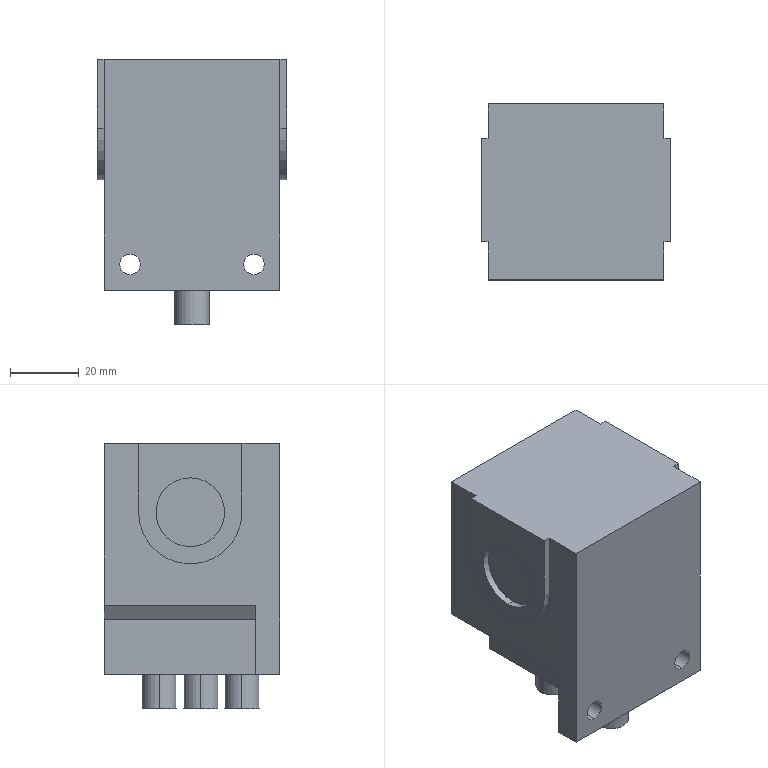Part | STEP file | Limit Switch | 1 solid | 40 faces | box 55 x 51 x 77 mm | volume 154232 mm3 | plane 23 | cylinder 17 | commonest cylinder face diameters 10 x6 6 x4 20 x4 30 x3
STEP:
#1=CARTESIAN_POINT('',(-18.,7.,-7.241));
#2=VERTEX_POINT('',#1);
#3=CARTESIAN_POINT('',(-18.,7.,-13.241));
#4=VERTEX_POINT('',#3);
#5=CARTESIAN_POINT('',(-18.,7.,-10.241));
#6=DIRECTION('',(0.,-1.,0.));
#7=DIRECTION('',(0.,0.,-1.));
#8=AXIS2_PLACEMENT_3D('',#5,#6,#7);
#9=CIRCLE('',#8,3.);
#10=EDGE_CURVE('',#2,#4,#9,.T.);
#11=ORIENTED_EDGE('',*,*,#10,.F.);
#12=CARTESIAN_POINT('',(-18.,0.,-7.241));
#13=VERTEX_POINT('',#12);
#14=CARTESIAN_POINT('',(-18.,44.,-7.241));
#15=DIRECTION('',(0.,-1.,0.));
#16=VECTOR('',#15,1000.);
#17=LINE('',#14,#16);
#18=EDGE_CURVE('',#2,#13,#17,.T.);
#19=ORIENTED_EDGE('',*,*,#18,.T.);
#20=CARTESIAN_POINT('',(-18.,0.,-13.241));
#21=VERTEX_POINT('',#20);
#22=CARTESIAN_POINT('',(-18.,0.,-10.241));
#23=DIRECTION('',(0.,-1.,0.));
#24=DIRECTION('',(0.,0.,-1.));
#25=AXIS2_PLACEMENT_3D('',#22,#23,#24);
#26=CIRCLE('',#25,3.);
#27=EDGE_CURVE('',#13,#21,#26,.T.);
#28=ORIENTED_EDGE('',*,*,#27,.T.);
#29=CARTESIAN_POINT('',(-18.,44.,-13.241));
#30=DIRECTION('',(0.,-1.,0.));
#31=VECTOR('',#30,1000.);
#32=LINE('',#29,#31);
#33=EDGE_CURVE('',#4,#21,#32,.T.);
#34=ORIENTED_EDGE('',*,*,#33,.F.);
#35=EDGE_LOOP('',(#11,#19,#28,#34));
#36=FACE_OUTER_BOUND('',#35,.T.);
#37=CARTESIAN_POINT('',(-18.,44.,-10.241));
#38=DIRECTION('',(0.,-1.,0.));
#39=DIRECTION('',(0.,0.,-1.));
#40=AXIS2_PLACEMENT_3D('',#37,#38,#39);
#41=CYLINDRICAL_SURFACE('',#40,3.);
#42=ADVANCED_FACE('',(#36),#41,.F.);
#43=CARTESIAN_POINT('',(18.,7.,-7.241));
#44=VERTEX_POINT('',#43);
#45=CARTESIAN_POINT('',(18.,7.,-13.241));
#46=VERTEX_POINT('',#45);
#47=CARTESIAN_POINT('',(18.,7.,-10.241));
#48=DIRECTION('',(0.,-1.,0.));
#49=DIRECTION('',(0.,0.,-1.));
#50=AXIS2_PLACEMENT_3D('',#47,#48,#49);
#51=CIRCLE('',#50,3.);
#52=EDGE_CURVE('',#44,#46,#51,.T.);
#53=ORIENTED_EDGE('',*,*,#52,.F.);
#54=CARTESIAN_POINT('',(18.,0.,-7.241));
#55=VERTEX_POINT('',#54);
#56=CARTESIAN_POINT('',(18.,44.,-7.241));
#57=DIRECTION('',(0.,-1.,0.));
#58=VECTOR('',#57,1000.);
#59=LINE('',#56,#58);
#60=EDGE_CURVE('',#44,#55,#59,.T.);
#61=ORIENTED_EDGE('',*,*,#60,.T.);
#62=CARTESIAN_POINT('',(18.,0.,-13.241));
#63=VERTEX_POINT('',#62);
#64=CARTESIAN_POINT('',(18.,0.,-10.241));
#65=DIRECTION('',(0.,-1.,0.));
#66=DIRECTION('',(0.,0.,-1.));
#67=AXIS2_PLACEMENT_3D('',#64,#65,#66);
#68=CIRCLE('',#67,3.);
#69=EDGE_CURVE('',#55,#63,#68,.T.);
#70=ORIENTED_EDGE('',*,*,#69,.T.);
#71=CARTESIAN_POINT('',(18.,44.,-13.241));
#72=DIRECTION('',(0.,-1.,0.));
#73=VECTOR('',#72,1000.);
#74=LINE('',#71,#73);
#75=EDGE_CURVE('',#46,#63,#74,.T.);
#76=ORIENTED_EDGE('',*,*,#75,.F.);
#77=EDGE_LOOP('',(#53,#61,#70,#76));
#78=FACE_OUTER_BOUND('',#77,.T.);
#79=CARTESIAN_POINT('',(18.,44.,-10.241));
#80=DIRECTION('',(0.,-1.,0.));
#81=DIRECTION('',(0.,0.,-1.));
#82=AXIS2_PLACEMENT_3D('',#79,#80,#81);
#83=CYLINDRICAL_SURFACE('',#82,3.);
#84=ADVANCED_FACE('',(#78),#83,.F.);
#85=CARTESIAN_POINT('',(-27.5,11.,29.259));
#86=VERTEX_POINT('',#85);
#87=CARTESIAN_POINT('',(-27.5,26.,14.259));
#88=VERTEX_POINT('',#87);
#89=CARTESIAN_POINT('',(-27.5,26.,29.259));
#90=DIRECTION('',(1.,0.,0.));
#91=DIRECTION('',(0.,0.,-1.));
#92=AXIS2_PLACEMENT_3D('',#89,#90,#91);
#93=CIRCLE('',#92,15.);
#94=EDGE_CURVE('',#86,#88,#93,.T.);
#95=ORIENTED_EDGE('',*,*,#94,.T.);
#96=CARTESIAN_POINT('',(-25.5,26.,14.259));
#97=VERTEX_POINT('',#96);
#98=CARTESIAN_POINT('',(-27.5,26.,14.259));
#99=DIRECTION('',(1.,0.,0.));
#100=VECTOR('',#99,1000.);
#101=LINE('',#98,#100);
#102=EDGE_CURVE('',#88,#97,#101,.T.);
#103=ORIENTED_EDGE('',*,*,#102,.T.);
#104=CARTESIAN_POINT('',(-25.5,11.,29.259));
#105=VERTEX_POINT('',#104);
#106=CARTESIAN_POINT('',(-25.5,26.,29.259));
#107=DIRECTION('',(-1.,0.,0.));
#108=DIRECTION('',(0.,0.,-1.));
#109=AXIS2_PLACEMENT_3D('',#106,#107,#108);
#110=CIRCLE('',#109,15.);
#111=EDGE_CURVE('',#97,#105,#110,.T.);
#112=ORIENTED_EDGE('',*,*,#111,.T.);
#113=CARTESIAN_POINT('',(-27.5,11.,29.259));
#114=DIRECTION('',(-1.,0.,0.));
#115=VECTOR('',#114,1000.);
#116=LINE('',#113,#115);
#117=EDGE_CURVE('',#105,#86,#116,.T.);
#118=ORIENTED_EDGE('',*,*,#117,.T.);
#119=EDGE_LOOP('',(#95,#103,#112,#118));
#120=FACE_OUTER_BOUND('',#119,.T.);
#121=CARTESIAN_POINT('',(-27.5,26.,29.259));
#122=DIRECTION('',(1.,0.,0.));
#123=DIRECTION('',(0.,0.,-1.));
#124=AXIS2_PLACEMENT_3D('',#121,#122,#123);
#125=CYLINDRICAL_SURFACE('',#124,15.);
#126=ADVANCED_FACE('',(#120),#125,.T.);
#127=CARTESIAN_POINT('',(5.,11.,-27.741));
#128=VERTEX_POINT('',#127);
#129=CARTESIAN_POINT('',(-5.,11.,-27.741));
#130=VERTEX_POINT('',#129);
#131=CARTESIAN_POINT('',(0.,11.,-27.741));
#132=DIRECTION('',(0.,0.,1.));
#133=DIRECTION('',(1.,0.,0.));
#134=AXIS2_PLACEMENT_3D('',#131,#132,#133);
#135=CIRCLE('',#134,5.);
#136=EDGE_CURVE('',#128,#130,#135,.T.);
#137=ORIENTED_EDGE('',*,*,#136,.T.);
#138=CARTESIAN_POINT('',(-5.,11.,-17.741));
#139=VERTEX_POINT('',#138);
#140=CARTESIAN_POINT('',(-5.,11.,-27.741));
#141=DIRECTION('',(0.,0.,1.));
#142=VECTOR('',#141,1000.);
#143=LINE('',#140,#142);
#144=EDGE_CURVE('',#130,#139,#143,.T.);
#145=ORIENTED_EDGE('',*,*,#144,.T.);
#146=CARTESIAN_POINT('',(5.,11.,-17.741));
#147=VERTEX_POINT('',#146);
#148=CARTESIAN_POINT('',(0.,11.,-17.741));
#149=DIRECTION('',(0.,0.,-1.));
#150=DIRECTION('',(1.,0.,0.));
#151=AXIS2_PLACEMENT_3D('',#148,#149,#150);
#152=CIRCLE('',#151,5.);
#153=EDGE_CURVE('',#139,#147,#152,.T.);
#154=ORIENTED_EDGE('',*,*,#153,.T.);
#155=CARTESIAN_POINT('',(5.,11.,-27.741));
#156=DIRECTION('',(0.,0.,1.));
#157=VECTOR('',#156,1000.);
#158=LINE('',#155,#157);
#159=EDGE_CURVE('',#128,#147,#158,.T.);
#160=ORIENTED_EDGE('',*,*,#159,.F.);
#161=EDGE_LOOP('',(#137,#145,#154,#160));
#162=FACE_OUTER_BOUND('',#161,.T.);
#163=CARTESIAN_POINT('',(0.,11.,-27.741));
#164=DIRECTION('',(0.,0.,1.));
#165=DIRECTION('',(1.,0.,0.));
#166=AXIS2_PLACEMENT_3D('',#163,#164,#165);
#167=CYLINDRICAL_SURFACE('',#166,5.);
#168=ADVANCED_FACE('',(#162),#167,.T.);
#169=CARTESIAN_POINT('',(5.,35.,-27.741));
#170=VERTEX_POINT('',#169);
#171=CARTESIAN_POINT('',(-5.,35.,-27.741));
#172=VERTEX_POINT('',#171);
#173=CARTESIAN_POINT('',(0.,35.,-27.741));
#174=DIRECTION('',(0.,0.,1.));
#175=DIRECTION('',(1.,0.,0.));
#176=AXIS2_PLACEMENT_3D('',#173,#174,#175);
#177=CIRCLE('',#176,5.);
#178=EDGE_CURVE('',#170,#172,#177,.T.);
#179=ORIENTED_EDGE('',*,*,#178,.T.);
#180=CARTESIAN_POINT('',(-5.,35.,-17.741));
#181=VERTEX_POINT('',#180);
#182=CARTESIAN_POINT('',(-5.,35.,-27.741));
#183=DIRECTION('',(0.,0.,1.));
#184=VECTOR('',#183,1000.);
#185=LINE('',#182,#184);
#186=EDGE_CURVE('',#172,#181,#185,.T.);
#187=ORIENTED_EDGE('',*,*,#186,.T.);
#188=CARTESIAN_POINT('',(5.,35.,-17.741));
#189=VERTEX_POINT('',#188);
#190=CARTESIAN_POINT('',(0.,35.,-17.741));
#191=DIRECTION('',(0.,0.,-1.));
#192=DIRECTION('',(1.,0.,0.));
#193=AXIS2_PLACEMENT_3D('',#190,#191,#192);
#194=CIRCLE('',#193,5.);
#195=EDGE_CURVE('',#181,#189,#194,.T.);
#196=ORIENTED_EDGE('',*,*,#195,.T.);
#197=CARTESIAN_POINT('',(5.,35.,-27.741));
#198=DIRECTION('',(0.,0.,1.));
#199=VECTOR('',#198,1000.);
#200=LINE('',#197,#199);
#201=EDGE_CURVE('',#170,#189,#200,.T.);
#202=ORIENTED_EDGE('',*,*,#201,.F.);
#203=EDGE_LOOP('',(#179,#187,#196,#202));
#204=FACE_OUTER_BOUND('',#203,.T.);
#205=CARTESIAN_POINT('',(0.,35.,-27.741));
#206=DIRECTION('',(0.,0.,1.));
#207=DIRECTION('',(1.,0.,0.));
#208=AXIS2_PLACEMENT_3D('',#205,#206,#207);
#209=CYLINDRICAL_SURFACE('',#208,5.);
#210=ADVANCED_FACE('',(#204),#209,.T.);
#211=CARTESIAN_POINT('',(5.,23.,-27.741));
#212=VERTEX_POINT('',#211);
#213=CARTESIAN_POINT('',(-5.,23.,-27.741));
#214=VERTEX_POINT('',#213);
#215=CARTESIAN_POINT('',(0.,23.,-27.741));
#216=DIRECTION('',(0.,0.,1.));
#217=DIRECTION('',(1.,0.,0.));
#218=AXIS2_PLACEMENT_3D('',#215,#216,#217);
#219=CIRCLE('',#218,5.);
#220=EDGE_CURVE('',#212,#214,#219,.T.);
#221=ORIENTED_EDGE('',*,*,#220,.T.);
#222=CARTESIAN_POINT('',(-5.,23.,-17.741));
#223=VERTEX_POINT('',#222);
#224=CARTESIAN_POINT('',(-5.,23.,-27.741));
#225=DIRECTION('',(0.,0.,1.));
#226=VECTOR('',#225,1000.);
#227=LINE('',#224,#226);
#228=EDGE_CURVE('',#214,#223,#227,.T.);
#229=ORIENTED_EDGE('',*,*,#228,.T.);
#230=CARTESIAN_POINT('',(5.,23.,-17.741));
#231=VERTEX_POINT('',#230);
#232=CARTESIAN_POINT('',(0.,23.,-17.741));
#233=DIRECTION('',(0.,0.,-1.));
#234=DIRECTION('',(1.,0.,0.));
#235=AXIS2_PLACEMENT_3D('',#232,#233,#234);
#236=CIRCLE('',#235,5.);
#237=EDGE_CURVE('',#223,#231,#236,.T.);
#238=ORIENTED_EDGE('',*,*,#237,.T.);
#239=CARTESIAN_POINT('',(5.,23.,-27.741));
#240=DIRECTION('',(0.,0.,1.));
#241=VECTOR('',#240,1000.);
#242=LINE('',#239,#241);
#243=EDGE_CURVE('',#212,#231,#242,.T.);
#244=ORIENTED_EDGE('',*,*,#243,.F.);
#245=EDGE_LOOP('',(#221,#229,#238,#244));
#246=FACE_OUTER_BOUND('',#245,.T.);
#247=CARTESIAN_POINT('',(0.,23.,-27.741));
#248=DIRECTION('',(0.,0.,1.));
#249=DIRECTION('',(1.,0.,0.));
#250=AXIS2_PLACEMENT_3D('',#247,#248,#249);
#251=CYLINDRICAL_SURFACE('',#250,5.);
#252=ADVANCED_FACE('',(#246),#251,.T.);
#253=CARTESIAN_POINT('',(27.5,26.,19.259));
#254=VERTEX_POINT('',#253);
#255=CARTESIAN_POINT('',(27.5,26.,39.259));
#256=VERTEX_POINT('',#255);
#257=CARTESIAN_POINT('',(27.5,26.,29.259));
#258=DIRECTION('',(-1.,0.,0.));
#259=DIRECTION('',(0.,0.,1.));
#260=AXIS2_PLACEMENT_3D('',#257,#258,#259);
#261=CIRCLE('',#260,10.);
#262=EDGE_CURVE('',#254,#256,#261,.T.);
#263=ORIENTED_EDGE('',*,*,#262,.F.);
#264=CARTESIAN_POINT('',(25.5,26.,19.259));
#265=VERTEX_POINT('',#264);
#266=CARTESIAN_POINT('',(27.5,26.,19.259));
#267=DIRECTION('',(-1.,0.,0.));
#268=VECTOR('',#267,1000.);
#269=LINE('',#266,#268);
#270=EDGE_CURVE('',#254,#265,#269,.T.);
#271=ORIENTED_EDGE('',*,*,#270,.T.);
#272=CARTESIAN_POINT('',(25.5,26.,39.259));
#273=VERTEX_POINT('',#272);
#274=CARTESIAN_POINT('',(25.5,26.,29.259));
#275=DIRECTION('',(1.,0.,0.));
#276=DIRECTION('',(0.,0.,1.));
#277=AXIS2_PLACEMENT_3D('',#274,#275,#276);
#278=CIRCLE('',#277,10.);
#279=EDGE_CURVE('',#273,#265,#278,.T.);
#280=ORIENTED_EDGE('',*,*,#279,.F.);
#281=CARTESIAN_POINT('',(27.5,26.,39.259));
#282=DIRECTION('',(-1.,0.,0.));
#283=VECTOR('',#282,1000.);
#284=LINE('',#281,#283);
#285=EDGE_CURVE('',#256,#273,#284,.T.);
#286=ORIENTED_EDGE('',*,*,#285,.F.);
#287=EDGE_LOOP('',(#263,#271,#280,#286));
#288=FACE_OUTER_BOUND('',#287,.T.);
#289=CARTESIAN_POINT('',(27.5,26.,29.259));
#290=DIRECTION('',(-1.,0.,0.));
#291=DIRECTION('',(0.,0.,1.));
#292=AXIS2_PLACEMENT_3D('',#289,#290,#291);
#293=CYLINDRICAL_SURFACE('',#292,10.);
#294=ADVANCED_FACE('',(#288),#293,.F.);
#295=CARTESIAN_POINT('',(-27.5,26.,39.259));
#296=VERTEX_POINT('',#295);
#297=CARTESIAN_POINT('',(-27.5,26.,19.259));
#298=VERTEX_POINT('',#297);
#299=CARTESIAN_POINT('',(-27.5,26.,29.259));
#300=DIRECTION('',(1.,0.,0.));
#301=DIRECTION('',(0.,0.,-1.));
#302=AXIS2_PLACEMENT_3D('',#299,#300,#301);
#303=CIRCLE('',#302,10.);
#304=EDGE_CURVE('',#296,#298,#303,.T.);
#305=ORIENTED_EDGE('',*,*,#304,.F.);
#306=CARTESIAN_POINT('',(-25.5,26.,39.259));
#307=VERTEX_POINT('',#306);
#308=CARTESIAN_POINT('',(-27.5,26.,39.259));
#309=DIRECTION('',(1.,0.,0.));
#310=VECTOR('',#309,1000.);
#311=LINE('',#308,#310);
#312=EDGE_CURVE('',#296,#307,#311,.T.);
#313=ORIENTED_EDGE('',*,*,#312,.T.);
#314=CARTESIAN_POINT('',(-25.5,26.,19.259));
#315=VERTEX_POINT('',#314);
#316=CARTESIAN_POINT('',(-25.5,26.,29.259));
#317=DIRECTION('',(-1.,0.,0.));
#318=DIRECTION('',(0.,0.,-1.));
#319=AXIS2_PLACEMENT_3D('',#316,#317,#318);
#320=CIRCLE('',#319,10.);
#321=EDGE_CURVE('',#315,#307,#320,.T.);
#322=ORIENTED_EDGE('',*,*,#321,.F.);
#323=CARTESIAN_POINT('',(-27.5,26.,19.259));
#324=DIRECTION('',(1.,0.,0.));
#325=VECTOR('',#324,1000.);
#326=LINE('',#323,#325);
#327=EDGE_CURVE('',#298,#315,#326,.T.);
#328=ORIENTED_EDGE('',*,*,#327,.F.);
#329=EDGE_LOOP('',(#305,#313,#322,#328));
#330=FACE_OUTER_BOUND('',#329,.T.);
#331=CARTESIAN_POINT('',(-27.5,26.,29.259));
#332=DIRECTION('',(1.,0.,0.));
#333=DIRECTION('',(0.,0.,-1.));
#334=AXIS2_PLACEMENT_3D('',#331,#332,#333);
#335=CYLINDRICAL_SURFACE('',#334,10.);
#336=ADVANCED_FACE('',(#330),#335,.F.);
#337=CARTESIAN_POINT('',(25.5,0.,-17.741));
#338=VERTEX_POINT('',#337);
#339=CARTESIAN_POINT('',(-25.5,0.,-17.741));
#340=VERTEX_POINT('',#339);
#341=CARTESIAN_POINT('',(0.,0.,-17.741));
#342=DIRECTION('',(-1.,0.,0.));
#343=VECTOR('',#342,1000.);
#344=LINE('',#341,#343);
#345=EDGE_CURVE('',#338,#340,#344,.T.);
#346=ORIENTED_EDGE('',*,*,#345,.F.);
#347=CARTESIAN_POINT('',(25.5,0.,49.259));
#348=VERTEX_POINT('',#347);
#349=CARTESIAN_POINT('',(25.5,0.,0.));
#350=DIRECTION('',(0.,0.,-1.));
#351=VECTOR('',#350,1000.);
#352=LINE('',#349,#351);
#353=EDGE_CURVE('',#348,#338,#352,.T.);
#354=ORIENTED_EDGE('',*,*,#353,.F.);
#355=CARTESIAN_POINT('',(-25.5,0.,49.259));
#356=VERTEX_POINT('',#355);
#357=CARTESIAN_POINT('',(0.,0.,49.259));
#358=DIRECTION('',(1.,0.,0.));
#359=VECTOR('',#358,1000.);
#360=LINE('',#357,#359);
#361=EDGE_CURVE('',#356,#348,#360,.T.);
#362=ORIENTED_EDGE('',*,*,#361,.F.);
#363=CARTESIAN_POINT('',(-25.5,0.,0.));
#364=DIRECTION('',(0.,0.,1.));
#365=VECTOR('',#364,1000.);
#366=LINE('',#363,#365);
#367=EDGE_CURVE('',#340,#356,#366,.T.);
#368=ORIENTED_EDGE('',*,*,#367,.F.);
#369=EDGE_LOOP('',(#346,#354,#362,#368));
#370=FACE_OUTER_BOUND('',#369,.T.);
#371=CARTESIAN_POINT('',(-18.,0.,-10.241));
#372=DIRECTION('',(0.,-1.,0.));
#373=DIRECTION('',(0.,0.,-1.));
#374=AXIS2_PLACEMENT_3D('',#371,#372,#373);
#375=CIRCLE('',#374,3.);
#376=EDGE_CURVE('',#21,#13,#375,.T.);
#377=ORIENTED_EDGE('',*,*,#376,.F.);
#378=ORIENTED_EDGE('',*,*,#27,.F.);
#379=EDGE_LOOP('',(#377,#378));
#380=FACE_BOUND('',#379,.T.);
#381=CARTESIAN_POINT('',(18.,0.,-10.241));
#382=DIRECTION('',(0.,-1.,0.));
#383=DIRECTION('',(0.,0.,-1.));
#384=AXIS2_PLACEMENT_3D('',#381,#382,#383);
#385=CIRCLE('',#384,3.);
#386=EDGE_CURVE('',#63,#55,#385,.T.);
#387=ORIENTED_EDGE('',*,*,#386,.F.);
#388=ORIENTED_EDGE('',*,*,#69,.F.);
#389=EDGE_LOOP('',(#387,#388));
#390=FACE_BOUND('',#389,.T.);
#391=CARTESIAN_POINT('',(0.,0.,0.));
#392=DIRECTION('',(0.,1.,0.));
#393=DIRECTION('',(0.,0.,1.));
#394=AXIS2_PLACEMENT_3D('',#391,#392,#393);
#395=PLANE('',#394);
#396=ADVANCED_FACE('',(#370,#380,#390),#395,.F.);
#397=CARTESIAN_POINT('',(-25.5,41.,29.259));
#398=VERTEX_POINT('',#397);
#399=CARTESIAN_POINT('',(-25.5,26.,29.259));
#400=DIRECTION('',(-1.,0.,0.));
#401=DIRECTION('',(0.,0.,-1.));
#402=AXIS2_PLACEMENT_3D('',#399,#400,#401);
#403=CIRCLE('',#402,15.);
#404=EDGE_CURVE('',#398,#97,#403,.T.);
#405=ORIENTED_EDGE('',*,*,#404,.F.);
#406=CARTESIAN_POINT('',(-25.5,41.,49.259));
#407=VERTEX_POINT('',#406);
#408=CARTESIAN_POINT('',(-25.5,41.,-17.741));
#409=DIRECTION('',(0.,0.,-1.));
#410=VECTOR('',#409,1000.);
#411=LINE('',#408,#410);
#412=EDGE_CURVE('',#407,#398,#411,.T.);
#413=ORIENTED_EDGE('',*,*,#412,.F.);
#414=CARTESIAN_POINT('',(-25.5,51.,49.259));
#415=VERTEX_POINT('',#414);
#416=CARTESIAN_POINT('',(-25.5,51.,49.259));
#417=DIRECTION('',(0.,-1.,0.));
#418=VECTOR('',#417,1000.);
#419=LINE('',#416,#418);
#420=EDGE_CURVE('',#415,#407,#419,.T.);
#421=ORIENTED_EDGE('',*,*,#420,.F.);
#422=CARTESIAN_POINT('',(-25.5,51.,2.259));
#423=VERTEX_POINT('',#422);
#424=CARTESIAN_POINT('',(-25.5,51.,-17.741));
#425=DIRECTION('',(0.,0.,1.));
#426=VECTOR('',#425,1000.);
#427=LINE('',#424,#426);
#428=EDGE_CURVE('',#423,#415,#427,.T.);
#429=ORIENTED_EDGE('',*,*,#428,.F.);
#430=CARTESIAN_POINT('',(-25.5,7.,2.259));
#431=VERTEX_POINT('',#430);
#432=CARTESIAN_POINT('',(-25.5,51.,2.259));
#433=DIRECTION('',(0.,1.,0.));
#434=VECTOR('',#433,1000.);
#435=LINE('',#432,#434);
#436=EDGE_CURVE('',#431,#423,#435,.T.);
#437=ORIENTED_EDGE('',*,*,#436,.F.);
#438=CARTESIAN_POINT('',(-25.5,7.,-17.741));
#439=VERTEX_POINT('',#438);
#440=CARTESIAN_POINT('',(-25.5,7.,-17.741));
#441=DIRECTION('',(0.,0.,1.));
#442=VECTOR('',#441,1000.);
#443=LINE('',#440,#442);
#444=EDGE_CURVE('',#439,#431,#443,.T.);
#445=ORIENTED_EDGE('',*,*,#444,.F.);
#446=CARTESIAN_POINT('',(-25.5,51.,-17.741));
#447=DIRECTION('',(0.,1.,0.));
#448=VECTOR('',#447,1000.);
#449=LINE('',#446,#448);
#450=EDGE_CURVE('',#340,#439,#449,.T.);
#451=ORIENTED_EDGE('',*,*,#450,.F.);
#452=ORIENTED_EDGE('',*,*,#367,.T.);
#453=CARTESIAN_POINT('',(-25.5,11.,49.259));
#454=VERTEX_POINT('',#453);
#455=CARTESIAN_POINT('',(-25.5,51.,49.259));
#456=DIRECTION('',(0.,-1.,0.));
#457=VECTOR('',#456,1000.);
#458=LINE('',#455,#457);
#459=EDGE_CURVE('',#454,#356,#458,.T.);
#460=ORIENTED_EDGE('',*,*,#459,.F.);
#461=CARTESIAN_POINT('',(-25.5,11.,-17.741));
#462=DIRECTION('',(0.,0.,1.));
#463=VECTOR('',#462,1000.);
#464=LINE('',#461,#463);
#465=EDGE_CURVE('',#105,#454,#464,.T.);
#466=ORIENTED_EDGE('',*,*,#465,.F.);
#467=ORIENTED_EDGE('',*,*,#111,.F.);
#468=EDGE_LOOP('',(#405,#413,#421,#429,#437,#445,#451,#452,#460,#466,#467));
#469=FACE_OUTER_BOUND('',#468,.T.);
#470=CARTESIAN_POINT('',(-25.5,51.,-17.741));
#471=DIRECTION('',(1.,0.,0.));
#472=DIRECTION('',(0.,0.,-1.));
#473=AXIS2_PLACEMENT_3D('',#470,#471,#472);
#474=PLANE('',#473);
#475=ADVANCED_FACE('',(#469),#474,.F.);
#476=CARTESIAN_POINT('',(0.,11.,-17.741));
#477=DIRECTION('',(0.,0.,-1.));
#478=DIRECTION('',(1.,0.,0.));
#479=AXIS2_PLACEMENT_3D('',#476,#477,#478);
#480=CIRCLE('',#479,5.);
#481=EDGE_CURVE('',#147,#139,#480,.T.);
#482=ORIENTED_EDGE('',*,*,#481,.F.);
#483=ORIENTED_EDGE('',*,*,#153,.F.);
#484=EDGE_LOOP('',(#482,#483));
#485=FACE_BOUND('',#484,.T.);
#486=CARTESIAN_POINT('',(0.,35.,-17.741));
#487=DIRECTION('',(0.,0.,-1.));
#488=DIRECTION('',(1.,0.,0.));
#489=AXIS2_PLACEMENT_3D('',#486,#487,#488);
#490=CIRCLE('',#489,5.);
#491=EDGE_CURVE('',#189,#181,#490,.T.);
#492=ORIENTED_EDGE('',*,*,#491,.F.);
#493=ORIENTED_EDGE('',*,*,#195,.F.);
#494=EDGE_LOOP('',(#492,#493));
#495=FACE_BOUND('',#494,.T.);
#496=CARTESIAN_POINT('',(10.,7.,-17.741));
#497=VERTEX_POINT('',#496);
#498=CARTESIAN_POINT('',(10.,51.,-17.741));
#499=VERTEX_POINT('',#498);
#500=CARTESIAN_POINT('',(10.,51.,-17.741));
#501=DIRECTION('',(0.,1.,0.));
#502=VECTOR('',#501,1000.);
#503=LINE('',#500,#502);
#504=EDGE_CURVE('',#497,#499,#503,.T.);
#505=ORIENTED_EDGE('',*,*,#504,.F.);
#506=CARTESIAN_POINT('',(25.5,7.,-17.741));
#507=VERTEX_POINT('',#506);
#508=CARTESIAN_POINT('',(-25.5,7.,-17.741));
#509=DIRECTION('',(-1.,0.,0.));
#510=VECTOR('',#509,1000.);
#511=LINE('',#508,#510);
#512=EDGE_CURVE('',#507,#497,#511,.T.);
#513=ORIENTED_EDGE('',*,*,#512,.F.);
#514=CARTESIAN_POINT('',(25.5,51.,-17.741));
#515=DIRECTION('',(0.,1.,0.));
#516=VECTOR('',#515,1000.);
#517=LINE('',#514,#516);
#518=EDGE_CURVE('',#338,#507,#517,.T.);
#519=ORIENTED_EDGE('',*,*,#518,.F.);
#520=ORIENTED_EDGE('',*,*,#345,.T.);
#521=ORIENTED_EDGE('',*,*,#450,.T.);
#522=CARTESIAN_POINT('',(-10.,7.,-17.741));
#523=VERTEX_POINT('',#522);
#524=CARTESIAN_POINT('',(-25.5,7.,-17.741));
#525=DIRECTION('',(-1.,0.,0.));
#526=VECTOR('',#525,1000.);
#527=LINE('',#524,#526);
#528=EDGE_CURVE('',#523,#439,#527,.T.);
#529=ORIENTED_EDGE('',*,*,#528,.F.);
#530=CARTESIAN_POINT('',(-10.,51.,-17.741));
#531=VERTEX_POINT('',#530);
#532=CARTESIAN_POINT('',(-10.,51.,-17.741));
#533=DIRECTION('',(0.,-1.,0.));
#534=VECTOR('',#533,1000.);
#535=LINE('',#532,#534);
#536=EDGE_CURVE('',#531,#523,#535,.T.);
#537=ORIENTED_EDGE('',*,*,#536,.F.);
#538=CARTESIAN_POINT('',(-25.5,51.,-17.741));
#539=DIRECTION('',(-1.,0.,0.));
#540=VECTOR('',#539,1000.);
#541=LINE('',#538,#540);
#542=EDGE_CURVE('',#499,#531,#541,.T.);
#543=ORIENTED_EDGE('',*,*,#542,.F.);
#544=EDGE_LOOP('',(#505,#513,#519,#520,#521,#529,#537,#543));
#545=FACE_OUTER_BOUND('',#544,.T.);
#546=CARTESIAN_POINT('',(0.,23.,-17.741));
#547=DIRECTION('',(0.,0.,-1.));
#548=DIRECTION('',(1.,0.,0.));
#549=AXIS2_PLACEMENT_3D('',#546,#547,#548);
#550=CIRCLE('',#549,5.);
#551=EDGE_CURVE('',#231,#223,#550,.T.);
#552=ORIENTED_EDGE('',*,*,#551,.F.);
#553=ORIENTED_EDGE('',*,*,#237,.F.);
#554=EDGE_LOOP('',(#552,#553));
#555=FACE_BOUND('',#554,.T.);
#556=CARTESIAN_POINT('',(-25.5,51.,-17.741));
#557=DIRECTION('',(0.,0.,1.));
#558=DIRECTION('',(1.,0.,0.));
#559=AXIS2_PLACEMENT_3D('',#556,#557,#558);
#560=PLANE('',#559);
#561=ADVANCED_FACE('',(#485,#495,#545,#555),#560,.F.);
#562=CARTESIAN_POINT('',(25.5,11.,49.259));
#563=VERTEX_POINT('',#562);
#564=CARTESIAN_POINT('',(25.5,51.,49.259));
#565=DIRECTION('',(0.,1.,0.));
#566=VECTOR('',#565,1000.);
#567=LINE('',#564,#566);
#568=EDGE_CURVE('',#348,#563,#567,.T.);
#569=ORIENTED_EDGE('',*,*,#568,.F.);
#570=ORIENTED_EDGE('',*,*,#353,.T.);
#571=ORIENTED_EDGE('',*,*,#518,.T.);
#572=CARTESIAN_POINT('',(25.5,7.,2.259));
#573=VERTEX_POINT('',#572);
#574=CARTESIAN_POINT('',(25.5,7.,-17.741));
#575=DIRECTION('',(0.,0.,-1.));
#576=VECTOR('',#575,1000.);
#577=LINE('',#574,#576);
#578=EDGE_CURVE('',#573,#507,#577,.T.);
#579=ORIENTED_EDGE('',*,*,#578,.F.);
#580=CARTESIAN_POINT('',(25.5,51.,2.259));
#581=VERTEX_POINT('',#580);
#582=CARTESIAN_POINT('',(25.5,51.,2.259));
#583=DIRECTION('',(0.,-1.,0.));
#584=VECTOR('',#583,1000.);
#585=LINE('',#582,#584);
#586=EDGE_CURVE('',#581,#573,#585,.T.);
#587=ORIENTED_EDGE('',*,*,#586,.F.);
#588=CARTESIAN_POINT('',(25.5,51.,49.259));
#589=VERTEX_POINT('',#588);
#590=CARTESIAN_POINT('',(25.5,51.,-17.741));
#591=DIRECTION('',(0.,0.,-1.));
#592=VECTOR('',#591,1000.);
#593=LINE('',#590,#592);
#594=EDGE_CURVE('',#589,#581,#593,.T.);
#595=ORIENTED_EDGE('',*,*,#594,.F.);
#596=CARTESIAN_POINT('',(25.5,41.,49.259));
#597=VERTEX_POINT('',#596);
#598=CARTESIAN_POINT('',(25.5,51.,49.259));
#599=DIRECTION('',(0.,1.,0.));
#600=VECTOR('',#599,1000.);
#601=LINE('',#598,#600);
#602=EDGE_CURVE('',#597,#589,#601,.T.);
#603=ORIENTED_EDGE('',*,*,#602,.F.);
#604=CARTESIAN_POINT('',(25.5,41.,29.259));
#605=VERTEX_POINT('',#604);
#606=CARTESIAN_POINT('',(25.5,41.,-17.741));
#607=DIRECTION('',(0.,0.,1.));
#608=VECTOR('',#607,1000.);
#609=LINE('',#606,#608);
#610=EDGE_CURVE('',#605,#597,#609,.T.);
#611=ORIENTED_EDGE('',*,*,#610,.F.);
#612=CARTESIAN_POINT('',(25.5,11.,29.259));
#613=VERTEX_POINT('',#612);
#614=CARTESIAN_POINT('',(25.5,26.,29.259));
#615=DIRECTION('',(1.,0.,0.));
#616=DIRECTION('',(0.,0.,1.));
#617=AXIS2_PLACEMENT_3D('',#614,#615,#616);
#618=CIRCLE('',#617,15.);
#619=EDGE_CURVE('',#613,#605,#618,.T.);
#620=ORIENTED_EDGE('',*,*,#619,.F.);
#621=CARTESIAN_POINT('',(25.5,11.,-17.741));
#622=DIRECTION('',(0.,0.,-1.));
#623=VECTOR('',#622,1000.);
#624=LINE('',#621,#623);
#625=EDGE_CURVE('',#563,#613,#624,.T.);
#626=ORIENTED_EDGE('',*,*,#625,.F.);
#627=EDGE_LOOP('',(#569,#570,#571,#579,#587,#595,#603,#611,#620,#626));
#628=FACE_OUTER_BOUND('',#627,.T.);
#629=CARTESIAN_POINT('',(25.5,51.,-17.741));
#630=DIRECTION('',(-1.,0.,0.));
#631=DIRECTION('',(0.,0.,1.));
#632=AXIS2_PLACEMENT_3D('',#629,#630,#631);
#633=PLANE('',#632);
#634=ADVANCED_FACE('',(#628),#633,.F.);
#635=ORIENTED_EDGE('',*,*,#568,.T.);
#636=CARTESIAN_POINT('',(27.5,11.,49.259));
#637=VERTEX_POINT('',#636);
#638=CARTESIAN_POINT('',(-25.5,11.,49.259));
#639=DIRECTION('',(-1.,0.,0.));
#640=VECTOR('',#639,1000.);
#641=LINE('',#638,#640);
#642=EDGE_CURVE('',#637,#563,#641,.T.);
#643=ORIENTED_EDGE('',*,*,#642,.F.);
#644=CARTESIAN_POINT('',(27.5,41.,49.259));
#645=VERTEX_POINT('',#644);
#646=CARTESIAN_POINT('',(27.5,51.,49.259));
#647=DIRECTION('',(0.,-1.,0.));
#648=VECTOR('',#647,1000.);
#649=LINE('',#646,#648);
#650=EDGE_CURVE('',#645,#637,#649,.T.);
#651=ORIENTED_EDGE('',*,*,#650,.F.);
#652=CARTESIAN_POINT('',(-25.5,41.,49.259));
#653=DIRECTION('',(1.,0.,0.));
#654=VECTOR('',#653,1000.);
#655=LINE('',#652,#654);
#656=EDGE_CURVE('',#597,#645,#655,.T.);
#657=ORIENTED_EDGE('',*,*,#656,.F.);
#658=ORIENTED_EDGE('',*,*,#602,.T.);
#659=CARTESIAN_POINT('',(-25.5,51.,49.259));
#660=DIRECTION('',(1.,0.,0.));
#661=VECTOR('',#660,1000.);
#662=LINE('',#659,#661);
#663=EDGE_CURVE('',#415,#589,#662,.T.);
#664=ORIENTED_EDGE('',*,*,#663,.F.);
#665=ORIENTED_EDGE('',*,*,#420,.T.);
#666=CARTESIAN_POINT('',(-27.5,41.,49.259));
#667=VERTEX_POINT('',#666);
#668=CARTESIAN_POINT('',(-25.5,41.,49.259));
#669=DIRECTION('',(1.,0.,0.));
#670=VECTOR('',#669,1000.);
#671=LINE('',#668,#670);
#672=EDGE_CURVE('',#667,#407,#671,.T.);
#673=ORIENTED_EDGE('',*,*,#672,.F.);
#674=CARTESIAN_POINT('',(-27.5,11.,49.259));
#675=VERTEX_POINT('',#674);
#676=CARTESIAN_POINT('',(-27.5,51.,49.259));
#677=DIRECTION('',(0.,1.,0.));
#678=VECTOR('',#677,1000.);
#679=LINE('',#676,#678);
#680=EDGE_CURVE('',#675,#667,#679,.T.);
#681=ORIENTED_EDGE('',*,*,#680,.F.);
#682=CARTESIAN_POINT('',(-25.5,11.,49.259));
#683=DIRECTION('',(-1.,0.,0.));
#684=VECTOR('',#683,1000.);
#685=LINE('',#682,#684);
#686=EDGE_CURVE('',#454,#675,#685,.T.);
#687=ORIENTED_EDGE('',*,*,#686,.F.);
#688=ORIENTED_EDGE('',*,*,#459,.T.);
#689=ORIENTED_EDGE('',*,*,#361,.T.);
#690=EDGE_LOOP('',(#635,#643,#651,#657,#658,#664,#665,#673,#681,#687,#688,#689));
#691=FACE_OUTER_BOUND('',#690,.T.);
#692=CARTESIAN_POINT('',(-25.5,51.,49.259));
#693=DIRECTION('',(0.,0.,-1.));
#694=DIRECTION('',(-1.,0.,0.));
#695=AXIS2_PLACEMENT_3D('',#692,#693,#694);
#696=PLANE('',#695);
#697=ADVANCED_FACE('',(#691),#696,.F.);
#698=ORIENTED_EDGE('',*,*,#18,.F.);
#699=CARTESIAN_POINT('',(-18.,7.,-10.241));
#700=DIRECTION('',(0.,-1.,0.));
#701=DIRECTION('',(0.,0.,-1.));
#702=AXIS2_PLACEMENT_3D('',#699,#700,#701);
#703=CIRCLE('',#702,3.);
#704=EDGE_CURVE('',#4,#2,#703,.T.);
#705=ORIENTED_EDGE('',*,*,#704,.F.);
#706=ORIENTED_EDGE('',*,*,#33,.T.);
#707=ORIENTED_EDGE('',*,*,#376,.T.);
#708=EDGE_LOOP('',(#698,#705,#706,#707));
#709=FACE_OUTER_BOUND('',#708,.T.);
#710=CARTESIAN_POINT('',(-18.,44.,-10.241));
#711=DIRECTION('',(0.,-1.,0.));
#712=DIRECTION('',(0.,0.,-1.));
#713=AXIS2_PLACEMENT_3D('',#710,#711,#712);
#714=CYLINDRICAL_SURFACE('',#713,3.);
#715=ADVANCED_FACE('',(#709),#714,.F.);
#716=ORIENTED_EDGE('',*,*,#60,.F.);
#717=CARTESIAN_POINT('',(18.,7.,-10.241));
#718=DIRECTION('',(0.,-1.,0.));
#719=DIRECTION('',(0.,0.,-1.));
#720=AXIS2_PLACEMENT_3D('',#717,#718,#719);
#721=CIRCLE('',#720,3.);
#722=EDGE_CURVE('',#46,#44,#721,.T.);
#723=ORIENTED_EDGE('',*,*,#722,.F.);
#724=ORIENTED_EDGE('',*,*,#75,.T.);
#725=ORIENTED_EDGE('',*,*,#386,.T.);
#726=EDGE_LOOP('',(#716,#723,#724,#725));
#727=FACE_OUTER_BOUND('',#726,.T.);
#728=CARTESIAN_POINT('',(18.,44.,-10.241));
#729=DIRECTION('',(0.,-1.,0.));
#730=DIRECTION('',(0.,0.,-1.));
#731=AXIS2_PLACEMENT_3D('',#728,#729,#730);
#732=CYLINDRICAL_SURFACE('',#731,3.);
#733=ADVANCED_FACE('',(#727),#732,.F.);
#734=ORIENTED_EDGE('',*,*,#102,.F.);
#735=CARTESIAN_POINT('',(-27.5,41.,29.259));
#736=VERTEX_POINT('',#735);
#737=CARTESIAN_POINT('',(-27.5,26.,29.259));
#738=DIRECTION('',(1.,0.,0.));
#739=DIRECTION('',(0.,0.,-1.));
#740=AXIS2_PLACEMENT_3D('',#737,#738,#739);
#741=CIRCLE('',#740,15.);
#742=EDGE_CURVE('',#88,#736,#741,.T.);
#743=ORIENTED_EDGE('',*,*,#742,.T.);
#744=CARTESIAN_POINT('',(-27.5,41.,29.259));
#745=DIRECTION('',(1.,0.,0.));
#746=VECTOR('',#745,1000.);
#747=LINE('',#744,#746);
#748=EDGE_CURVE('',#736,#398,#747,.T.);
#749=ORIENTED_EDGE('',*,*,#748,.T.);
#750=ORIENTED_EDGE('',*,*,#404,.T.);
#751=EDGE_LOOP('',(#734,#743,#749,#750));
#752=FACE_OUTER_BOUND('',#751,.T.);
#753=CARTESIAN_POINT('',(-27.5,26.,29.259));
#754=DIRECTION('',(1.,0.,0.));
#755=DIRECTION('',(0.,0.,-1.));
#756=AXIS2_PLACEMENT_3D('',#753,#754,#755);
#757=CYLINDRICAL_SURFACE('',#756,15.);
#758=ADVANCED_FACE('',(#752),#757,.T.);
#759=CARTESIAN_POINT('',(-27.5,41.,29.259));
#760=DIRECTION('',(0.,0.,1.));
#761=VECTOR('',#760,1000.);
#762=LINE('',#759,#761);
#763=EDGE_CURVE('',#736,#667,#762,.T.);
#764=ORIENTED_EDGE('',*,*,#763,.T.);
#765=ORIENTED_EDGE('',*,*,#672,.T.);
#766=ORIENTED_EDGE('',*,*,#412,.T.);
#767=ORIENTED_EDGE('',*,*,#748,.F.);
#768=EDGE_LOOP('',(#764,#765,#766,#767));
#769=FACE_OUTER_BOUND('',#768,.T.);
#770=CARTESIAN_POINT('',(-27.5,41.,29.259));
#771=DIRECTION('',(0.,1.,0.));
#772=DIRECTION('',(0.,0.,1.));
#773=AXIS2_PLACEMENT_3D('',#770,#771,#772);
#774=PLANE('',#773);
#775=ADVANCED_FACE('',(#769),#774,.T.);
#776=ORIENTED_EDGE('',*,*,#663,.T.);
#777=ORIENTED_EDGE('',*,*,#594,.T.);
#778=CARTESIAN_POINT('',(10.,51.,-1.741));
#779=VERTEX_POINT('',#778);
#780=CARTESIAN_POINT('',(25.5,51.,2.259));
#781=DIRECTION('',(-0.9683,0.,-0.2499));
#782=VECTOR('',#781,1000.);
#783=LINE('',#780,#782);
#784=EDGE_CURVE('',#581,#779,#783,.T.);
#785=ORIENTED_EDGE('',*,*,#784,.T.);
#786=CARTESIAN_POINT('',(10.,51.,0.));
#787=DIRECTION('',(0.,0.,-1.));
#788=VECTOR('',#787,1000.);
#789=LINE('',#786,#788);
#790=EDGE_CURVE('',#779,#499,#789,.T.);
#791=ORIENTED_EDGE('',*,*,#790,.T.);
#792=ORIENTED_EDGE('',*,*,#542,.T.);
#793=CARTESIAN_POINT('',(-10.,51.,-1.741));
#794=VERTEX_POINT('',#793);
#795=CARTESIAN_POINT('',(-10.,51.,0.));
#796=DIRECTION('',(0.,0.,1.));
#797=VECTOR('',#796,1000.);
#798=LINE('',#795,#797);
#799=EDGE_CURVE('',#531,#794,#798,.T.);
#800=ORIENTED_EDGE('',*,*,#799,.T.);
#801=CARTESIAN_POINT('',(-10.,51.,-1.741));
#802=DIRECTION('',(-0.9683,0.,0.2499));
#803=VECTOR('',#802,1000.);
#804=LINE('',#801,#803);
#805=EDGE_CURVE('',#794,#423,#804,.T.);
#806=ORIENTED_EDGE('',*,*,#805,.T.);
#807=ORIENTED_EDGE('',*,*,#428,.T.);
#808=EDGE_LOOP('',(#776,#777,#785,#791,#792,#800,#806,#807));
#809=FACE_OUTER_BOUND('',#808,.T.);
#810=CARTESIAN_POINT('',(0.,51.,0.));
#811=DIRECTION('',(0.,1.,0.));
#812=DIRECTION('',(0.,0.,1.));
#813=AXIS2_PLACEMENT_3D('',#810,#811,#812);
#814=PLANE('',#813);
#815=ADVANCED_FACE('',(#809),#814,.T.);
#816=CARTESIAN_POINT('',(-10.,7.,-1.741));
#817=VERTEX_POINT('',#816);
#818=CARTESIAN_POINT('',(-10.,7.,-1.741));
#819=DIRECTION('',(0.,1.,0.));
#820=VECTOR('',#819,1000.);
#821=LINE('',#818,#820);
#822=EDGE_CURVE('',#817,#794,#821,.T.);
#823=ORIENTED_EDGE('',*,*,#822,.F.);
#824=CARTESIAN_POINT('',(-10.,7.,-1.741));
#825=DIRECTION('',(0.9683,0.,-0.2499));
#826=VECTOR('',#825,1000.);
#827=LINE('',#824,#826);
#828=EDGE_CURVE('',#431,#817,#827,.T.);
#829=ORIENTED_EDGE('',*,*,#828,.F.);
#830=ORIENTED_EDGE('',*,*,#436,.T.);
#831=ORIENTED_EDGE('',*,*,#805,.F.);
#832=EDGE_LOOP('',(#823,#829,#830,#831));
#833=FACE_OUTER_BOUND('',#832,.T.);
#834=CARTESIAN_POINT('',(-10.,7.,-1.741));
#835=DIRECTION('',(0.2499,0.,0.9683));
#836=DIRECTION('',(0.9683,0.,-0.2499));
#837=AXIS2_PLACEMENT_3D('',#834,#835,#836);
#838=PLANE('',#837);
#839=ADVANCED_FACE('',(#833),#838,.F.);
#840=ORIENTED_EDGE('',*,*,#444,.T.);
#841=ORIENTED_EDGE('',*,*,#828,.T.);
#842=CARTESIAN_POINT('',(-10.,7.,0.));
#843=DIRECTION('',(0.,0.,1.));
#844=VECTOR('',#843,1000.);
#845=LINE('',#842,#844);
#846=EDGE_CURVE('',#523,#817,#845,.T.);
#847=ORIENTED_EDGE('',*,*,#846,.F.);
#848=ORIENTED_EDGE('',*,*,#528,.T.);
#849=EDGE_LOOP('',(#840,#841,#847,#848));
#850=FACE_OUTER_BOUND('',#849,.T.);
#851=ORIENTED_EDGE('',*,*,#704,.T.);
#852=ORIENTED_EDGE('',*,*,#10,.T.);
#853=EDGE_LOOP('',(#851,#852));
#854=FACE_BOUND('',#853,.T.);
#855=CARTESIAN_POINT('',(0.,7.,0.));
#856=DIRECTION('',(0.,-1.,0.));
#857=DIRECTION('',(0.,0.,-1.));
#858=AXIS2_PLACEMENT_3D('',#855,#856,#857);
#859=PLANE('',#858);
#860=ADVANCED_FACE('',(#850,#854),#859,.F.);
#861=CARTESIAN_POINT('',(-27.5,11.,29.259));
#862=DIRECTION('',(0.,0.,-1.));
#863=VECTOR('',#862,1000.);
#864=LINE('',#861,#863);
#865=EDGE_CURVE('',#675,#86,#864,.T.);
#866=ORIENTED_EDGE('',*,*,#865,.T.);
#867=ORIENTED_EDGE('',*,*,#117,.F.);
#868=ORIENTED_EDGE('',*,*,#465,.T.);
#869=ORIENTED_EDGE('',*,*,#686,.T.);
#870=EDGE_LOOP('',(#866,#867,#868,#869));
#871=FACE_OUTER_BOUND('',#870,.T.);
#872=CARTESIAN_POINT('',(-27.5,11.,29.259));
#873=DIRECTION('',(0.,-1.,0.));
#874=DIRECTION('',(0.,0.,-1.));
#875=AXIS2_PLACEMENT_3D('',#872,#873,#874);
#876=PLANE('',#875);
#877=ADVANCED_FACE('',(#871),#876,.T.);
#878=ORIENTED_EDGE('',*,*,#144,.F.);
#879=CARTESIAN_POINT('',(0.,11.,-27.741));
#880=DIRECTION('',(0.,0.,1.));
#881=DIRECTION('',(1.,0.,0.));
#882=AXIS2_PLACEMENT_3D('',#879,#880,#881);
#883=CIRCLE('',#882,5.);
#884=EDGE_CURVE('',#130,#128,#883,.T.);
#885=ORIENTED_EDGE('',*,*,#884,.T.);
#886=ORIENTED_EDGE('',*,*,#159,.T.);
#887=ORIENTED_EDGE('',*,*,#481,.T.);
#888=EDGE_LOOP('',(#878,#885,#886,#887));
#889=FACE_OUTER_BOUND('',#888,.T.);
#890=CARTESIAN_POINT('',(0.,11.,-27.741));
#891=DIRECTION('',(0.,0.,1.));
#892=DIRECTION('',(1.,0.,0.));
#893=AXIS2_PLACEMENT_3D('',#890,#891,#892);
#894=CYLINDRICAL_SURFACE('',#893,5.);
#895=ADVANCED_FACE('',(#889),#894,.T.);
#896=ORIENTED_EDGE('',*,*,#186,.F.);
#897=CARTESIAN_POINT('',(0.,35.,-27.741));
#898=DIRECTION('',(0.,0.,1.));
#899=DIRECTION('',(1.,0.,0.));
#900=AXIS2_PLACEMENT_3D('',#897,#898,#899);
#901=CIRCLE('',#900,5.);
#902=EDGE_CURVE('',#172,#170,#901,.T.);
#903=ORIENTED_EDGE('',*,*,#902,.T.);
#904=ORIENTED_EDGE('',*,*,#201,.T.);
#905=ORIENTED_EDGE('',*,*,#491,.T.);
#906=EDGE_LOOP('',(#896,#903,#904,#905));
#907=FACE_OUTER_BOUND('',#906,.T.);
#908=CARTESIAN_POINT('',(0.,35.,-27.741));
#909=DIRECTION('',(0.,0.,1.));
#910=DIRECTION('',(1.,0.,0.));
#911=AXIS2_PLACEMENT_3D('',#908,#909,#910);
#912=CYLINDRICAL_SURFACE('',#911,5.);
#913=ADVANCED_FACE('',(#907),#912,.T.);
#914=CARTESIAN_POINT('',(10.,7.,-1.741));
#915=VERTEX_POINT('',#914);
#916=CARTESIAN_POINT('',(10.,7.,-1.741));
#917=DIRECTION('',(0.,1.,0.));
#918=VECTOR('',#917,1000.);
#919=LINE('',#916,#918);
#920=EDGE_CURVE('',#915,#779,#919,.T.);
#921=ORIENTED_EDGE('',*,*,#920,.F.);
#922=CARTESIAN_POINT('',(10.,7.,-17.741));
#923=DIRECTION('',(0.,0.,1.));
#924=VECTOR('',#923,1000.);
#925=LINE('',#922,#924);
#926=EDGE_CURVE('',#497,#915,#925,.T.);
#927=ORIENTED_EDGE('',*,*,#926,.F.);
#928=ORIENTED_EDGE('',*,*,#504,.T.);
#929=ORIENTED_EDGE('',*,*,#790,.F.);
#930=EDGE_LOOP('',(#921,#927,#928,#929));
#931=FACE_OUTER_BOUND('',#930,.T.);
#932=CARTESIAN_POINT('',(10.,7.,-17.741));
#933=DIRECTION('',(-1.,0.,0.));
#934=DIRECTION('',(0.,0.,1.));
#935=AXIS2_PLACEMENT_3D('',#932,#933,#934);
#936=PLANE('',#935);
#937=ADVANCED_FACE('',(#931),#936,.F.);
#938=ORIENTED_EDGE('',*,*,#926,.T.);
#939=CARTESIAN_POINT('',(10.,7.,-1.741));
#940=DIRECTION('',(0.9683,0.,0.2499));
#941=VECTOR('',#940,1000.);
#942=LINE('',#939,#941);
#943=EDGE_CURVE('',#915,#573,#942,.T.);
#944=ORIENTED_EDGE('',*,*,#943,.T.);
#945=ORIENTED_EDGE('',*,*,#578,.T.);
#946=ORIENTED_EDGE('',*,*,#512,.T.);
#947=EDGE_LOOP('',(#938,#944,#945,#946));
#948=FACE_OUTER_BOUND('',#947,.T.);
#949=ORIENTED_EDGE('',*,*,#722,.T.);
#950=ORIENTED_EDGE('',*,*,#52,.T.);
#951=EDGE_LOOP('',(#949,#950));
#952=FACE_BOUND('',#951,.T.);
#953=CARTESIAN_POINT('',(0.,7.,0.));
#954=DIRECTION('',(0.,1.,0.));
#955=DIRECTION('',(0.,0.,1.));
#956=AXIS2_PLACEMENT_3D('',#953,#954,#955);
#957=PLANE('',#956);
#958=ADVANCED_FACE('',(#948,#952),#957,.T.);
#959=ORIENTED_EDGE('',*,*,#536,.T.);
#960=ORIENTED_EDGE('',*,*,#846,.T.);
#961=ORIENTED_EDGE('',*,*,#822,.T.);
#962=ORIENTED_EDGE('',*,*,#799,.F.);
#963=EDGE_LOOP('',(#959,#960,#961,#962));
#964=FACE_OUTER_BOUND('',#963,.T.);
#965=CARTESIAN_POINT('',(-10.,7.,-17.741));
#966=DIRECTION('',(1.,0.,0.));
#967=DIRECTION('',(0.,0.,-1.));
#968=AXIS2_PLACEMENT_3D('',#965,#966,#967);
#969=PLANE('',#968);
#970=ADVANCED_FACE('',(#964),#969,.F.);
#971=ORIENTED_EDGE('',*,*,#228,.F.);
#972=CARTESIAN_POINT('',(0.,23.,-27.741));
#973=DIRECTION('',(0.,0.,1.));
#974=DIRECTION('',(1.,0.,0.));
#975=AXIS2_PLACEMENT_3D('',#972,#973,#974);
#976=CIRCLE('',#975,5.);
#977=EDGE_CURVE('',#214,#212,#976,.T.);
#978=ORIENTED_EDGE('',*,*,#977,.T.);
#979=ORIENTED_EDGE('',*,*,#243,.T.);
#980=ORIENTED_EDGE('',*,*,#551,.T.);
#981=EDGE_LOOP('',(#971,#978,#979,#980));
#982=FACE_OUTER_BOUND('',#981,.T.);
#983=CARTESIAN_POINT('',(0.,23.,-27.741));
#984=DIRECTION('',(0.,0.,1.));
#985=DIRECTION('',(1.,0.,0.));
#986=AXIS2_PLACEMENT_3D('',#983,#984,#985);
#987=CYLINDRICAL_SURFACE('',#986,5.);
#988=ADVANCED_FACE('',(#982),#987,.T.);
#989=CARTESIAN_POINT('',(27.5,11.,29.259));
#990=VERTEX_POINT('',#989);
#991=CARTESIAN_POINT('',(27.5,11.,29.259));
#992=DIRECTION('',(-1.,0.,0.));
#993=VECTOR('',#992,1000.);
#994=LINE('',#991,#993);
#995=EDGE_CURVE('',#990,#613,#994,.T.);
#996=ORIENTED_EDGE('',*,*,#995,.F.);
#997=CARTESIAN_POINT('',(27.5,11.,29.259));
#998=DIRECTION('',(0.,0.,-1.));
#999=VECTOR('',#998,1000.);
#1000=LINE('',#997,#999);
#1001=EDGE_CURVE('',#637,#990,#1000,.T.);
#1002=ORIENTED_EDGE('',*,*,#1001,.F.);
#1003=ORIENTED_EDGE('',*,*,#642,.T.);
#1004=ORIENTED_EDGE('',*,*,#625,.T.);
#1005=EDGE_LOOP('',(#996,#1002,#1003,#1004));
#1006=FACE_OUTER_BOUND('',#1005,.T.);
#1007=CARTESIAN_POINT('',(27.5,11.,29.259));
#1008=DIRECTION('',(0.,1.,0.));
#1009=DIRECTION('',(0.,0.,1.));
#1010=AXIS2_PLACEMENT_3D('',#1007,#1008,#1009);
#1011=PLANE('',#1010);
#1012=ADVANCED_FACE('',(#1006),#1011,.F.);
#1013=ORIENTED_EDGE('',*,*,#586,.T.);
#1014=ORIENTED_EDGE('',*,*,#943,.F.);
#1015=ORIENTED_EDGE('',*,*,#920,.T.);
#1016=ORIENTED_EDGE('',*,*,#784,.F.);
#1017=EDGE_LOOP('',(#1013,#1014,#1015,#1016));
#1018=FACE_OUTER_BOUND('',#1017,.T.);
#1019=CARTESIAN_POINT('',(10.,7.,-1.741));
#1020=DIRECTION('',(-0.2499,0.,0.9683));
#1021=DIRECTION('',(0.9683,0.,0.2499));
#1022=AXIS2_PLACEMENT_3D('',#1019,#1020,#1021);
#1023=PLANE('',#1022);
#1024=ADVANCED_FACE('',(#1018),#1023,.F.);
#1025=ORIENTED_EDGE('',*,*,#656,.T.);
#1026=CARTESIAN_POINT('',(27.5,41.,29.259));
#1027=VERTEX_POINT('',#1026);
#1028=CARTESIAN_POINT('',(27.5,41.,29.259));
#1029=DIRECTION('',(0.,0.,1.));
#1030=VECTOR('',#1029,1000.);
#1031=LINE('',#1028,#1030);
#1032=EDGE_CURVE('',#1027,#645,#1031,.T.);
#1033=ORIENTED_EDGE('',*,*,#1032,.F.);
#1034=CARTESIAN_POINT('',(27.5,41.,29.259));
#1035=DIRECTION('',(1.,0.,0.));
#1036=VECTOR('',#1035,1000.);
#1037=LINE('',#1034,#1036);
#1038=EDGE_CURVE('',#605,#1027,#1037,.T.);
#1039=ORIENTED_EDGE('',*,*,#1038,.F.);
#1040=ORIENTED_EDGE('',*,*,#610,.T.);
#1041=EDGE_LOOP('',(#1025,#1033,#1039,#1040));
#1042=FACE_OUTER_BOUND('',#1041,.T.);
#1043=CARTESIAN_POINT('',(27.5,41.,29.259));
#1044=DIRECTION('',(0.,-1.,0.));
#1045=DIRECTION('',(0.,0.,-1.));
#1046=AXIS2_PLACEMENT_3D('',#1043,#1044,#1045);
#1047=PLANE('',#1046);
#1048=ADVANCED_FACE('',(#1042),#1047,.F.);
#1049=CARTESIAN_POINT('',(27.5,26.,29.259));
#1050=DIRECTION('',(-1.,0.,0.));
#1051=DIRECTION('',(0.,0.,1.));
#1052=AXIS2_PLACEMENT_3D('',#1049,#1050,#1051);
#1053=CIRCLE('',#1052,15.);
#1054=EDGE_CURVE('',#1027,#990,#1053,.T.);
#1055=ORIENTED_EDGE('',*,*,#1054,.T.);
#1056=ORIENTED_EDGE('',*,*,#995,.T.);
#1057=ORIENTED_EDGE('',*,*,#619,.T.);
#1058=ORIENTED_EDGE('',*,*,#1038,.T.);
#1059=EDGE_LOOP('',(#1055,#1056,#1057,#1058));
#1060=FACE_OUTER_BOUND('',#1059,.T.);
#1061=CARTESIAN_POINT('',(27.5,26.,29.259));
#1062=DIRECTION('',(-1.,0.,0.));
#1063=DIRECTION('',(0.,0.,1.));
#1064=AXIS2_PLACEMENT_3D('',#1061,#1062,#1063);
#1065=CYLINDRICAL_SURFACE('',#1064,15.);
#1066=ADVANCED_FACE('',(#1060),#1065,.T.);
#1067=CARTESIAN_POINT('',(27.5,26.,29.259));
#1068=DIRECTION('',(-1.,0.,0.));
#1069=DIRECTION('',(0.,0.,1.));
#1070=AXIS2_PLACEMENT_3D('',#1067,#1068,#1069);
#1071=CIRCLE('',#1070,10.);
#1072=EDGE_CURVE('',#256,#254,#1071,.T.);
#1073=ORIENTED_EDGE('',*,*,#1072,.T.);
#1074=ORIENTED_EDGE('',*,*,#262,.T.);
#1075=EDGE_LOOP('',(#1073,#1074));
#1076=FACE_BOUND('',#1075,.T.);
#1077=ORIENTED_EDGE('',*,*,#650,.T.);
#1078=ORIENTED_EDGE('',*,*,#1001,.T.);
#1079=ORIENTED_EDGE('',*,*,#1054,.F.);
#1080=ORIENTED_EDGE('',*,*,#1032,.T.);
#1081=EDGE_LOOP('',(#1077,#1078,#1079,#1080));
#1082=FACE_OUTER_BOUND('',#1081,.T.);
#1083=CARTESIAN_POINT('',(27.5,26.,29.259));
#1084=DIRECTION('',(1.,0.,0.));
#1085=DIRECTION('',(0.,0.,-1.));
#1086=AXIS2_PLACEMENT_3D('',#1083,#1084,#1085);
#1087=PLANE('',#1086);
#1088=ADVANCED_FACE('',(#1076,#1082),#1087,.T.);
#1089=ORIENTED_EDGE('',*,*,#763,.F.);
#1090=ORIENTED_EDGE('',*,*,#742,.F.);
#1091=ORIENTED_EDGE('',*,*,#94,.F.);
#1092=ORIENTED_EDGE('',*,*,#865,.F.);
#1093=ORIENTED_EDGE('',*,*,#680,.T.);
#1094=EDGE_LOOP('',(#1089,#1090,#1091,#1092,#1093));
#1095=FACE_OUTER_BOUND('',#1094,.T.);
#1096=CARTESIAN_POINT('',(-27.5,26.,29.259));
#1097=DIRECTION('',(1.,0.,0.));
#1098=DIRECTION('',(0.,0.,-1.));
#1099=AXIS2_PLACEMENT_3D('',#1096,#1097,#1098);
#1100=CIRCLE('',#1099,10.);
#1101=EDGE_CURVE('',#298,#296,#1100,.T.);
#1102=ORIENTED_EDGE('',*,*,#1101,.T.);
#1103=ORIENTED_EDGE('',*,*,#304,.T.);
#1104=EDGE_LOOP('',(#1102,#1103));
#1105=FACE_BOUND('',#1104,.T.);
#1106=CARTESIAN_POINT('',(-27.5,26.,29.259));
#1107=DIRECTION('',(-1.,0.,0.));
#1108=DIRECTION('',(0.,0.,1.));
#1109=AXIS2_PLACEMENT_3D('',#1106,#1107,#1108);
#1110=PLANE('',#1109);
#1111=ADVANCED_FACE('',(#1095,#1105),#1110,.T.);
#1112=ORIENTED_EDGE('',*,*,#136,.F.);
#1113=ORIENTED_EDGE('',*,*,#884,.F.);
#1114=EDGE_LOOP('',(#1112,#1113));
#1115=FACE_OUTER_BOUND('',#1114,.T.);
#1116=CARTESIAN_POINT('',(0.,11.,-27.741));
#1117=DIRECTION('',(0.,0.,-1.));
#1118=DIRECTION('',(-1.,0.,0.));
#1119=AXIS2_PLACEMENT_3D('',#1116,#1117,#1118);
#1120=PLANE('',#1119);
#1121=ADVANCED_FACE('',(#1115),#1120,.T.);
#1122=ORIENTED_EDGE('',*,*,#178,.F.);
#1123=ORIENTED_EDGE('',*,*,#902,.F.);
#1124=EDGE_LOOP('',(#1122,#1123));
#1125=FACE_OUTER_BOUND('',#1124,.T.);
#1126=CARTESIAN_POINT('',(0.,35.,-27.741));
#1127=DIRECTION('',(0.,0.,-1.));
#1128=DIRECTION('',(-1.,0.,0.));
#1129=AXIS2_PLACEMENT_3D('',#1126,#1127,#1128);
#1130=PLANE('',#1129);
#1131=ADVANCED_FACE('',(#1125),#1130,.T.);
#1132=ORIENTED_EDGE('',*,*,#220,.F.);
#1133=ORIENTED_EDGE('',*,*,#977,.F.);
#1134=EDGE_LOOP('',(#1132,#1133));
#1135=FACE_OUTER_BOUND('',#1134,.T.);
#1136=CARTESIAN_POINT('',(0.,23.,-27.741));
#1137=DIRECTION('',(0.,0.,-1.));
#1138=DIRECTION('',(-1.,0.,0.));
#1139=AXIS2_PLACEMENT_3D('',#1136,#1137,#1138);
#1140=PLANE('',#1139);
#1141=ADVANCED_FACE('',(#1135),#1140,.T.);
#1142=ORIENTED_EDGE('',*,*,#270,.F.);
#1143=ORIENTED_EDGE('',*,*,#1072,.F.);
#1144=ORIENTED_EDGE('',*,*,#285,.T.);
#1145=CARTESIAN_POINT('',(25.5,26.,29.259));
#1146=DIRECTION('',(1.,0.,0.));
#1147=DIRECTION('',(0.,0.,1.));
#1148=AXIS2_PLACEMENT_3D('',#1145,#1146,#1147);
#1149=CIRCLE('',#1148,10.);
#1150=EDGE_CURVE('',#265,#273,#1149,.T.);
#1151=ORIENTED_EDGE('',*,*,#1150,.F.);
#1152=EDGE_LOOP('',(#1142,#1143,#1144,#1151));
#1153=FACE_OUTER_BOUND('',#1152,.T.);
#1154=CARTESIAN_POINT('',(27.5,26.,29.259));
#1155=DIRECTION('',(-1.,0.,0.));
#1156=DIRECTION('',(0.,0.,1.));
#1157=AXIS2_PLACEMENT_3D('',#1154,#1155,#1156);
#1158=CYLINDRICAL_SURFACE('',#1157,10.);
#1159=ADVANCED_FACE('',(#1153),#1158,.F.);
#1160=ORIENTED_EDGE('',*,*,#312,.F.);
#1161=ORIENTED_EDGE('',*,*,#1101,.F.);
#1162=ORIENTED_EDGE('',*,*,#327,.T.);
#1163=CARTESIAN_POINT('',(-25.5,26.,29.259));
#1164=DIRECTION('',(-1.,0.,0.));
#1165=DIRECTION('',(0.,0.,-1.));
#1166=AXIS2_PLACEMENT_3D('',#1163,#1164,#1165);
#1167=CIRCLE('',#1166,10.);
#1168=EDGE_CURVE('',#307,#315,#1167,.T.);
#1169=ORIENTED_EDGE('',*,*,#1168,.F.);
#1170=EDGE_LOOP('',(#1160,#1161,#1162,#1169));
#1171=FACE_OUTER_BOUND('',#1170,.T.);
#1172=CARTESIAN_POINT('',(-27.5,26.,29.259));
#1173=DIRECTION('',(1.,0.,0.));
#1174=DIRECTION('',(0.,0.,-1.));
#1175=AXIS2_PLACEMENT_3D('',#1172,#1173,#1174);
#1176=CYLINDRICAL_SURFACE('',#1175,10.);
#1177=ADVANCED_FACE('',(#1171),#1176,.F.);
#1178=ORIENTED_EDGE('',*,*,#279,.T.);
#1179=ORIENTED_EDGE('',*,*,#1150,.T.);
#1180=EDGE_LOOP('',(#1178,#1179));
#1181=FACE_OUTER_BOUND('',#1180,.T.);
#1182=CARTESIAN_POINT('',(25.5,51.,-17.741));
#1183=DIRECTION('',(-1.,0.,0.));
#1184=DIRECTION('',(0.,0.,1.));
#1185=AXIS2_PLACEMENT_3D('',#1182,#1183,#1184);
#1186=PLANE('',#1185);
#1187=ADVANCED_FACE('',(#1181),#1186,.F.);
#1188=ORIENTED_EDGE('',*,*,#321,.T.);
#1189=ORIENTED_EDGE('',*,*,#1168,.T.);
#1190=EDGE_LOOP('',(#1188,#1189));
#1191=FACE_OUTER_BOUND('',#1190,.T.);
#1192=CARTESIAN_POINT('',(-25.5,51.,-17.741));
#1193=DIRECTION('',(1.,0.,0.));
#1194=DIRECTION('',(0.,0.,-1.));
#1195=AXIS2_PLACEMENT_3D('',#1192,#1193,#1194);
#1196=PLANE('',#1195);
#1197=ADVANCED_FACE('',(#1191),#1196,.F.);
#1198=CLOSED_SHELL('',(#42,#84,#126,#168,#210,#252,#294,#336,#396,#475,#561,#634,#697,#715,#733,#758,#775,#815,#839,#860,#877,#895,#913,#937,#958,#970,#988,#1012,#1024,#1048,#1066,#1088,#1111,#1121,#1131,#1141,#1159,#1177,#1187,#1197));
#1199=MANIFOLD_SOLID_BREP('',#1198);
#1200=CARTESIAN_POINT('',(0.,0.,0.));
#1201=DIRECTION('',(0.,0.,1.));
#1202=DIRECTION('',(1.,0.,0.));
#1203=AXIS2_PLACEMENT_3D('',#1200,#1201,#1202);
#1204=(LENGTH_UNIT()NAMED_UNIT(*)SI_UNIT(.MILLI.,.METRE.));
#1205=UNCERTAINTY_MEASURE_WITH_UNIT(LENGTH_MEASURE(0.00001),#1204,'','');
#1206=(NAMED_UNIT(*)PLANE_ANGLE_UNIT()SI_UNIT($,.RADIAN.));
#1207=(NAMED_UNIT(*)SI_UNIT($,.STERADIAN.)SOLID_ANGLE_UNIT());
#1208=(GEOMETRIC_REPRESENTATION_CONTEXT(3)GLOBAL_UNCERTAINTY_ASSIGNED_CONTEXT((#1205))GLOBAL_UNIT_ASSIGNED_CONTEXT((#1204,#1206,#1207))REPRESENTATION_CONTEXT('',''));
#1209=ADVANCED_BREP_SHAPE_REPRESENTATION('',(#1199,#1203),#1208);